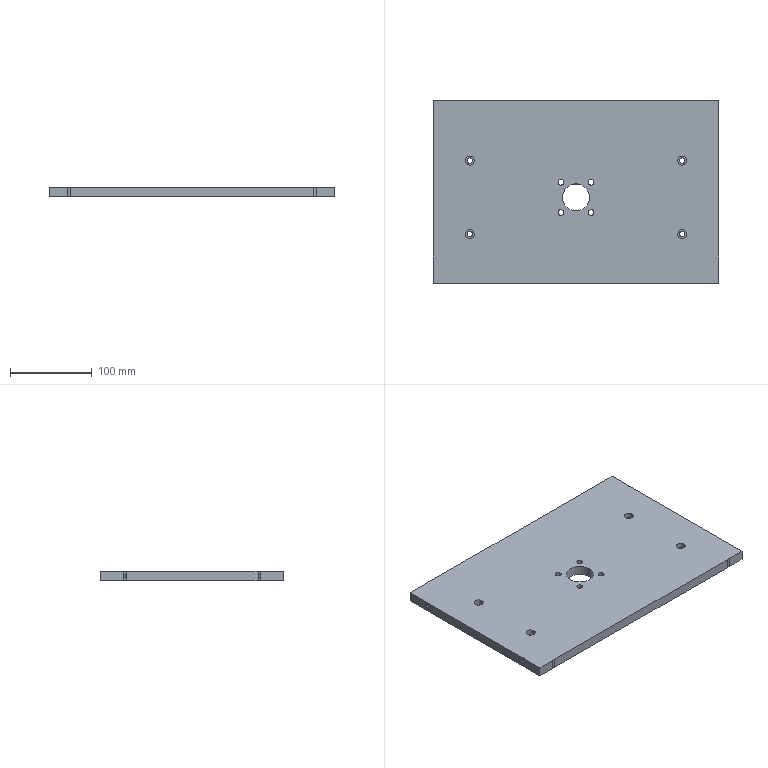Part | SolidWorks | features BaseBody 1 | 1 solid | 86 faces | box 350 x 225 x 12 mm | volume 928615 mm3 | cylinder 62 | plane 24 | commonest cylinder face diameters 3.3 x18 10 x18 6.6 x8 7 x8 11 x8 33 x2